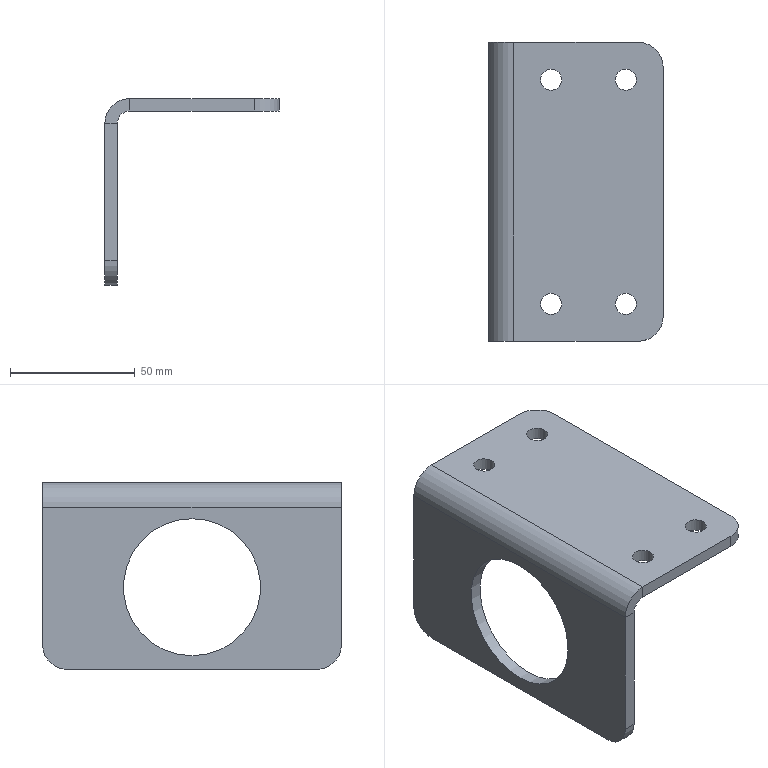Part | STEP file | JBJ-P-1007-02 | 1 solid | 23 faces | box 70 x 120 x 75 mm | volume 68625 mm3 | plane 12 | cylinder 11 | commonest cylinder face diameters 20 x5 8.5 x4 10 x1 55 x1
STEP:
#1=CARTESIAN_POINT('',(10.,-120.,75.));
#2=VERTEX_POINT('',#1);
#3=CARTESIAN_POINT('',(10.,-120.,70.));
#4=VERTEX_POINT('',#3);
#5=CARTESIAN_POINT('',(10.,-120.,75.));
#6=DIRECTION('',(0.,0.,-1.));
#7=VECTOR('',#6,1000.);
#8=LINE('',#5,#7);
#9=EDGE_CURVE('',#2,#4,#8,.T.);
#10=ORIENTED_EDGE('',*,*,#9,.F.);
#11=CARTESIAN_POINT('',(0.,-120.,65.));
#12=VERTEX_POINT('',#11);
#13=CARTESIAN_POINT('',(10.,-120.,65.));
#14=DIRECTION('',(0.,1.,0.));
#15=DIRECTION('',(0.,0.,-1.));
#16=AXIS2_PLACEMENT_3D('',#13,#14,#15);
#17=CIRCLE('',#16,10.);
#18=EDGE_CURVE('',#12,#2,#17,.T.);
#19=ORIENTED_EDGE('',*,*,#18,.F.);
#20=CARTESIAN_POINT('',(5.,-120.,65.));
#21=VERTEX_POINT('',#20);
#22=CARTESIAN_POINT('',(5.,-120.,65.));
#23=DIRECTION('',(-1.,0.,0.));
#24=VECTOR('',#23,1000.);
#25=LINE('',#22,#24);
#26=EDGE_CURVE('',#21,#12,#25,.T.);
#27=ORIENTED_EDGE('',*,*,#26,.F.);
#28=CARTESIAN_POINT('',(10.,-120.,65.));
#29=DIRECTION('',(0.,1.,0.));
#30=DIRECTION('',(1.,0.,0.));
#31=AXIS2_PLACEMENT_3D('',#28,#29,#30);
#32=CIRCLE('',#31,5.);
#33=EDGE_CURVE('',#21,#4,#32,.T.);
#34=ORIENTED_EDGE('',*,*,#33,.T.);
#35=EDGE_LOOP('',(#10,#19,#27,#34));
#36=FACE_OUTER_BOUND('',#35,.T.);
#37=CARTESIAN_POINT('',(10.,-120.,75.));
#38=DIRECTION('',(0.,-1.,0.));
#39=DIRECTION('',(0.,0.,-1.));
#40=AXIS2_PLACEMENT_3D('',#37,#38,#39);
#41=PLANE('',#40);
#42=ADVANCED_FACE('',(#36),#41,.T.);
#43=CARTESIAN_POINT('',(60.,-120.,70.));
#44=VERTEX_POINT('',#43);
#45=CARTESIAN_POINT('',(0.,-120.,70.));
#46=DIRECTION('',(1.,0.,0.));
#47=VECTOR('',#46,1000.);
#48=LINE('',#45,#47);
#49=EDGE_CURVE('',#4,#44,#48,.T.);
#50=ORIENTED_EDGE('',*,*,#49,.T.);
#51=CARTESIAN_POINT('',(60.,-120.,75.));
#52=VERTEX_POINT('',#51);
#53=CARTESIAN_POINT('',(60.,-120.,75.));
#54=DIRECTION('',(0.,0.,1.));
#55=VECTOR('',#54,1000.);
#56=LINE('',#53,#55);
#57=EDGE_CURVE('',#44,#52,#56,.T.);
#58=ORIENTED_EDGE('',*,*,#57,.T.);
#59=CARTESIAN_POINT('',(0.,-120.,75.));
#60=DIRECTION('',(1.,0.,0.));
#61=VECTOR('',#60,1000.);
#62=LINE('',#59,#61);
#63=EDGE_CURVE('',#2,#52,#62,.T.);
#64=ORIENTED_EDGE('',*,*,#63,.F.);
#65=ORIENTED_EDGE('',*,*,#9,.T.);
#66=EDGE_LOOP('',(#50,#58,#64,#65));
#67=FACE_OUTER_BOUND('',#66,.T.);
#68=CARTESIAN_POINT('',(5.,-120.,65.));
#69=DIRECTION('',(0.,-1.,0.));
#70=DIRECTION('',(0.,0.,-1.));
#71=AXIS2_PLACEMENT_3D('',#68,#69,#70);
#72=PLANE('',#71);
#73=ADVANCED_FACE('',(#67),#72,.T.);
#74=CARTESIAN_POINT('',(0.,0.,65.));
#75=VERTEX_POINT('',#74);
#76=CARTESIAN_POINT('',(5.,0.,65.));
#77=VERTEX_POINT('',#76);
#78=CARTESIAN_POINT('',(0.,0.,65.));
#79=DIRECTION('',(1.,0.,0.));
#80=VECTOR('',#79,1000.);
#81=LINE('',#78,#80);
#82=EDGE_CURVE('',#75,#77,#81,.T.);
#83=ORIENTED_EDGE('',*,*,#82,.F.);
#84=CARTESIAN_POINT('',(10.,0.,75.));
#85=VERTEX_POINT('',#84);
#86=CARTESIAN_POINT('',(10.,0.,65.));
#87=DIRECTION('',(0.,1.,0.));
#88=DIRECTION('',(0.,0.,-1.));
#89=AXIS2_PLACEMENT_3D('',#86,#87,#88);
#90=CIRCLE('',#89,10.);
#91=EDGE_CURVE('',#75,#85,#90,.T.);
#92=ORIENTED_EDGE('',*,*,#91,.T.);
#93=CARTESIAN_POINT('',(10.,0.,70.));
#94=VERTEX_POINT('',#93);
#95=CARTESIAN_POINT('',(10.,0.,70.));
#96=DIRECTION('',(0.,0.,1.));
#97=VECTOR('',#96,1000.);
#98=LINE('',#95,#97);
#99=EDGE_CURVE('',#94,#85,#98,.T.);
#100=ORIENTED_EDGE('',*,*,#99,.F.);
#101=CARTESIAN_POINT('',(10.,0.,65.));
#102=DIRECTION('',(0.,1.,0.));
#103=DIRECTION('',(1.,0.,0.));
#104=AXIS2_PLACEMENT_3D('',#101,#102,#103);
#105=CIRCLE('',#104,5.);
#106=EDGE_CURVE('',#77,#94,#105,.T.);
#107=ORIENTED_EDGE('',*,*,#106,.F.);
#108=EDGE_LOOP('',(#83,#92,#100,#107));
#109=FACE_OUTER_BOUND('',#108,.T.);
#110=CARTESIAN_POINT('',(0.,0.,65.));
#111=DIRECTION('',(0.,1.,0.));
#112=DIRECTION('',(0.,0.,1.));
#113=AXIS2_PLACEMENT_3D('',#110,#111,#112);
#114=PLANE('',#113);
#115=ADVANCED_FACE('',(#109),#114,.T.);
#116=CARTESIAN_POINT('',(5.,0.,10.));
#117=VERTEX_POINT('',#116);
#118=CARTESIAN_POINT('',(5.,0.,0.));
#119=DIRECTION('',(0.,0.,1.));
#120=VECTOR('',#119,1000.);
#121=LINE('',#118,#120);
#122=EDGE_CURVE('',#117,#77,#121,.T.);
#123=ORIENTED_EDGE('',*,*,#122,.F.);
#124=CARTESIAN_POINT('',(0.,0.,10.));
#125=VERTEX_POINT('',#124);
#126=CARTESIAN_POINT('',(0.,0.,10.));
#127=DIRECTION('',(-1.,0.,0.));
#128=VECTOR('',#127,1000.);
#129=LINE('',#126,#128);
#130=EDGE_CURVE('',#117,#125,#129,.T.);
#131=ORIENTED_EDGE('',*,*,#130,.T.);
#132=CARTESIAN_POINT('',(0.,0.,0.));
#133=DIRECTION('',(0.,0.,1.));
#134=VECTOR('',#133,1000.);
#135=LINE('',#132,#134);
#136=EDGE_CURVE('',#125,#75,#135,.T.);
#137=ORIENTED_EDGE('',*,*,#136,.T.);
#138=ORIENTED_EDGE('',*,*,#82,.T.);
#139=EDGE_LOOP('',(#123,#131,#137,#138));
#140=FACE_OUTER_BOUND('',#139,.T.);
#141=CARTESIAN_POINT('',(10.,0.,70.));
#142=DIRECTION('',(0.,1.,0.));
#143=DIRECTION('',(0.,0.,1.));
#144=AXIS2_PLACEMENT_3D('',#141,#142,#143);
#145=PLANE('',#144);
#146=ADVANCED_FACE('',(#140),#145,.T.);
#147=CARTESIAN_POINT('',(50.75,-15.,75.));
#148=VERTEX_POINT('',#147);
#149=CARTESIAN_POINT('',(55.,-15.,75.));
#150=DIRECTION('',(0.,0.,-1.));
#151=DIRECTION('',(-1.,0.,0.));
#152=AXIS2_PLACEMENT_3D('',#149,#150,#151);
#153=CIRCLE('',#152,4.25);
#154=EDGE_CURVE('',#148,#148,#153,.T.);
#155=ORIENTED_EDGE('',*,*,#154,.T.);
#156=EDGE_LOOP('',(#155));
#157=FACE_BOUND('',#156,.T.);
#158=CARTESIAN_POINT('',(20.75,-15.,75.));
#159=VERTEX_POINT('',#158);
#160=CARTESIAN_POINT('',(25.,-15.,75.));
#161=DIRECTION('',(0.,0.,-1.));
#162=DIRECTION('',(-1.,0.,0.));
#163=AXIS2_PLACEMENT_3D('',#160,#161,#162);
#164=CIRCLE('',#163,4.25);
#165=EDGE_CURVE('',#159,#159,#164,.T.);
#166=ORIENTED_EDGE('',*,*,#165,.T.);
#167=EDGE_LOOP('',(#166));
#168=FACE_BOUND('',#167,.T.);
#169=CARTESIAN_POINT('',(50.75,-105.,75.));
#170=VERTEX_POINT('',#169);
#171=CARTESIAN_POINT('',(55.,-105.,75.));
#172=DIRECTION('',(0.,0.,-1.));
#173=DIRECTION('',(-1.,0.,0.));
#174=AXIS2_PLACEMENT_3D('',#171,#172,#173);
#175=CIRCLE('',#174,4.25);
#176=EDGE_CURVE('',#170,#170,#175,.T.);
#177=ORIENTED_EDGE('',*,*,#176,.T.);
#178=EDGE_LOOP('',(#177));
#179=FACE_BOUND('',#178,.T.);
#180=CARTESIAN_POINT('',(20.75,-105.,75.));
#181=VERTEX_POINT('',#180);
#182=CARTESIAN_POINT('',(25.,-105.,75.));
#183=DIRECTION('',(0.,0.,-1.));
#184=DIRECTION('',(-1.,0.,0.));
#185=AXIS2_PLACEMENT_3D('',#182,#183,#184);
#186=CIRCLE('',#185,4.25);
#187=EDGE_CURVE('',#181,#181,#186,.T.);
#188=ORIENTED_EDGE('',*,*,#187,.T.);
#189=EDGE_LOOP('',(#188));
#190=FACE_BOUND('',#189,.T.);
#191=CARTESIAN_POINT('',(70.,-110.,75.));
#192=VERTEX_POINT('',#191);
#193=CARTESIAN_POINT('',(70.,-10.,75.));
#194=VERTEX_POINT('',#193);
#195=CARTESIAN_POINT('',(70.,-120.,75.));
#196=DIRECTION('',(0.,1.,0.));
#197=VECTOR('',#196,1000.);
#198=LINE('',#195,#197);
#199=EDGE_CURVE('',#192,#194,#198,.T.);
#200=ORIENTED_EDGE('',*,*,#199,.T.);
#201=CARTESIAN_POINT('',(60.,0.,75.));
#202=VERTEX_POINT('',#201);
#203=CARTESIAN_POINT('',(60.,-10.,75.));
#204=DIRECTION('',(0.,0.,1.));
#205=DIRECTION('',(1.,0.,0.));
#206=AXIS2_PLACEMENT_3D('',#203,#204,#205);
#207=CIRCLE('',#206,10.);
#208=EDGE_CURVE('',#194,#202,#207,.T.);
#209=ORIENTED_EDGE('',*,*,#208,.T.);
#210=CARTESIAN_POINT('',(0.,0.,75.));
#211=DIRECTION('',(1.,0.,0.));
#212=VECTOR('',#211,1000.);
#213=LINE('',#210,#212);
#214=EDGE_CURVE('',#85,#202,#213,.T.);
#215=ORIENTED_EDGE('',*,*,#214,.F.);
#216=CARTESIAN_POINT('',(10.,-120.,75.));
#217=DIRECTION('',(0.,1.,0.));
#218=VECTOR('',#217,1000.);
#219=LINE('',#216,#218);
#220=EDGE_CURVE('',#2,#85,#219,.T.);
#221=ORIENTED_EDGE('',*,*,#220,.F.);
#222=ORIENTED_EDGE('',*,*,#63,.T.);
#223=CARTESIAN_POINT('',(60.,-110.,75.));
#224=DIRECTION('',(0.,0.,1.));
#225=DIRECTION('',(1.,0.,0.));
#226=AXIS2_PLACEMENT_3D('',#223,#224,#225);
#227=CIRCLE('',#226,10.);
#228=EDGE_CURVE('',#52,#192,#227,.T.);
#229=ORIENTED_EDGE('',*,*,#228,.T.);
#230=EDGE_LOOP('',(#200,#209,#215,#221,#222,#229));
#231=FACE_OUTER_BOUND('',#230,.T.);
#232=CARTESIAN_POINT('',(0.,-120.,75.));
#233=DIRECTION('',(0.,0.,1.));
#234=DIRECTION('',(1.,0.,0.));
#235=AXIS2_PLACEMENT_3D('',#232,#233,#234);
#236=PLANE('',#235);
#237=ADVANCED_FACE('',(#157,#168,#179,#190,#231),#236,.T.);
#238=ORIENTED_EDGE('',*,*,#91,.F.);
#239=CARTESIAN_POINT('',(0.,-120.,65.));
#240=DIRECTION('',(0.,1.,0.));
#241=VECTOR('',#240,1000.);
#242=LINE('',#239,#241);
#243=EDGE_CURVE('',#12,#75,#242,.T.);
#244=ORIENTED_EDGE('',*,*,#243,.F.);
#245=ORIENTED_EDGE('',*,*,#18,.T.);
#246=ORIENTED_EDGE('',*,*,#220,.T.);
#247=EDGE_LOOP('',(#238,#244,#245,#246));
#248=FACE_OUTER_BOUND('',#247,.T.);
#249=CARTESIAN_POINT('',(10.,-120.,65.));
#250=DIRECTION('',(0.,1.,0.));
#251=DIRECTION('',(0.,0.,1.));
#252=AXIS2_PLACEMENT_3D('',#249,#250,#251);
#253=CYLINDRICAL_SURFACE('',#252,10.);
#254=ADVANCED_FACE('',(#248),#253,.T.);
#255=CARTESIAN_POINT('',(0.,-60.,5.5));
#256=VERTEX_POINT('',#255);
#257=CARTESIAN_POINT('',(0.,-60.,33.));
#258=DIRECTION('',(1.,0.,0.));
#259=DIRECTION('',(0.,0.,-1.));
#260=AXIS2_PLACEMENT_3D('',#257,#258,#259);
#261=CIRCLE('',#260,27.5);
#262=EDGE_CURVE('',#256,#256,#261,.T.);
#263=ORIENTED_EDGE('',*,*,#262,.T.);
#264=EDGE_LOOP('',(#263));
#265=FACE_BOUND('',#264,.T.);
#266=CARTESIAN_POINT('',(0.,-110.,0.));
#267=VERTEX_POINT('',#266);
#268=CARTESIAN_POINT('',(0.,-10.,0.));
#269=VERTEX_POINT('',#268);
#270=CARTESIAN_POINT('',(0.,-120.,0.));
#271=DIRECTION('',(0.,1.,0.));
#272=VECTOR('',#271,1000.);
#273=LINE('',#270,#272);
#274=EDGE_CURVE('',#267,#269,#273,.T.);
#275=ORIENTED_EDGE('',*,*,#274,.F.);
#276=CARTESIAN_POINT('',(0.,-120.,10.));
#277=VERTEX_POINT('',#276);
#278=CARTESIAN_POINT('',(0.,-110.,10.));
#279=DIRECTION('',(-1.,0.,0.));
#280=DIRECTION('',(0.,0.,1.));
#281=AXIS2_PLACEMENT_3D('',#278,#279,#280);
#282=CIRCLE('',#281,10.);
#283=EDGE_CURVE('',#267,#277,#282,.T.);
#284=ORIENTED_EDGE('',*,*,#283,.T.);
#285=CARTESIAN_POINT('',(0.,-120.,0.));
#286=DIRECTION('',(0.,0.,1.));
#287=VECTOR('',#286,1000.);
#288=LINE('',#285,#287);
#289=EDGE_CURVE('',#277,#12,#288,.T.);
#290=ORIENTED_EDGE('',*,*,#289,.T.);
#291=ORIENTED_EDGE('',*,*,#243,.T.);
#292=ORIENTED_EDGE('',*,*,#136,.F.);
#293=CARTESIAN_POINT('',(0.,-10.,10.));
#294=DIRECTION('',(-1.,0.,0.));
#295=DIRECTION('',(0.,0.,1.));
#296=AXIS2_PLACEMENT_3D('',#293,#294,#295);
#297=CIRCLE('',#296,10.);
#298=EDGE_CURVE('',#125,#269,#297,.T.);
#299=ORIENTED_EDGE('',*,*,#298,.T.);
#300=EDGE_LOOP('',(#275,#284,#290,#291,#292,#299));
#301=FACE_OUTER_BOUND('',#300,.T.);
#302=CARTESIAN_POINT('',(0.,-120.,0.));
#303=DIRECTION('',(-1.,0.,0.));
#304=DIRECTION('',(0.,0.,1.));
#305=AXIS2_PLACEMENT_3D('',#302,#303,#304);
#306=PLANE('',#305);
#307=ADVANCED_FACE('',(#265,#301),#306,.T.);
#308=CARTESIAN_POINT('',(5.,-110.,0.));
#309=VERTEX_POINT('',#308);
#310=CARTESIAN_POINT('',(5.,-10.,0.));
#311=VERTEX_POINT('',#310);
#312=CARTESIAN_POINT('',(5.,-120.,0.));
#313=DIRECTION('',(0.,1.,0.));
#314=VECTOR('',#313,1000.);
#315=LINE('',#312,#314);
#316=EDGE_CURVE('',#309,#311,#315,.T.);
#317=ORIENTED_EDGE('',*,*,#316,.F.);
#318=CARTESIAN_POINT('',(0.,-110.,0.));
#319=DIRECTION('',(-1.,0.,0.));
#320=VECTOR('',#319,1000.);
#321=LINE('',#318,#320);
#322=EDGE_CURVE('',#309,#267,#321,.T.);
#323=ORIENTED_EDGE('',*,*,#322,.T.);
#324=ORIENTED_EDGE('',*,*,#274,.T.);
#325=CARTESIAN_POINT('',(5.,-10.,0.));
#326=DIRECTION('',(1.,0.,0.));
#327=VECTOR('',#326,1000.);
#328=LINE('',#325,#327);
#329=EDGE_CURVE('',#269,#311,#328,.T.);
#330=ORIENTED_EDGE('',*,*,#329,.T.);
#331=EDGE_LOOP('',(#317,#323,#324,#330));
#332=FACE_OUTER_BOUND('',#331,.T.);
#333=CARTESIAN_POINT('',(0.,-120.,0.));
#334=DIRECTION('',(0.,0.,1.));
#335=DIRECTION('',(1.,0.,0.));
#336=AXIS2_PLACEMENT_3D('',#333,#334,#335);
#337=PLANE('',#336);
#338=ADVANCED_FACE('',(#332),#337,.F.);
#339=CARTESIAN_POINT('',(5.,-60.,5.5));
#340=VERTEX_POINT('',#339);
#341=CARTESIAN_POINT('',(5.,-60.,33.));
#342=DIRECTION('',(1.,0.,0.));
#343=DIRECTION('',(0.,0.,-1.));
#344=AXIS2_PLACEMENT_3D('',#341,#342,#343);
#345=CIRCLE('',#344,27.5);
#346=EDGE_CURVE('',#340,#340,#345,.T.);
#347=ORIENTED_EDGE('',*,*,#346,.F.);
#348=EDGE_LOOP('',(#347));
#349=FACE_BOUND('',#348,.T.);
#350=CARTESIAN_POINT('',(5.,-120.,10.));
#351=VERTEX_POINT('',#350);
#352=CARTESIAN_POINT('',(5.,-120.,0.));
#353=DIRECTION('',(0.,0.,1.));
#354=VECTOR('',#353,1000.);
#355=LINE('',#352,#354);
#356=EDGE_CURVE('',#351,#21,#355,.T.);
#357=ORIENTED_EDGE('',*,*,#356,.F.);
#358=CARTESIAN_POINT('',(5.,-110.,10.));
#359=DIRECTION('',(1.,0.,0.));
#360=DIRECTION('',(0.,0.,1.));
#361=AXIS2_PLACEMENT_3D('',#358,#359,#360);
#362=CIRCLE('',#361,10.);
#363=EDGE_CURVE('',#351,#309,#362,.T.);
#364=ORIENTED_EDGE('',*,*,#363,.T.);
#365=ORIENTED_EDGE('',*,*,#316,.T.);
#366=CARTESIAN_POINT('',(5.,-10.,10.));
#367=DIRECTION('',(1.,0.,0.));
#368=DIRECTION('',(0.,0.,1.));
#369=AXIS2_PLACEMENT_3D('',#366,#367,#368);
#370=CIRCLE('',#369,10.);
#371=EDGE_CURVE('',#311,#117,#370,.T.);
#372=ORIENTED_EDGE('',*,*,#371,.T.);
#373=ORIENTED_EDGE('',*,*,#122,.T.);
#374=CARTESIAN_POINT('',(5.,-120.,65.));
#375=DIRECTION('',(0.,1.,0.));
#376=VECTOR('',#375,1000.);
#377=LINE('',#374,#376);
#378=EDGE_CURVE('',#21,#77,#377,.T.);
#379=ORIENTED_EDGE('',*,*,#378,.F.);
#380=EDGE_LOOP('',(#357,#364,#365,#372,#373,#379));
#381=FACE_OUTER_BOUND('',#380,.T.);
#382=CARTESIAN_POINT('',(5.,-120.,0.));
#383=DIRECTION('',(-1.,0.,0.));
#384=DIRECTION('',(0.,0.,1.));
#385=AXIS2_PLACEMENT_3D('',#382,#383,#384);
#386=PLANE('',#385);
#387=ADVANCED_FACE('',(#349,#381),#386,.F.);
#388=ORIENTED_EDGE('',*,*,#106,.T.);
#389=CARTESIAN_POINT('',(10.,-120.,70.));
#390=DIRECTION('',(0.,1.,0.));
#391=VECTOR('',#390,1000.);
#392=LINE('',#389,#391);
#393=EDGE_CURVE('',#4,#94,#392,.T.);
#394=ORIENTED_EDGE('',*,*,#393,.F.);
#395=ORIENTED_EDGE('',*,*,#33,.F.);
#396=ORIENTED_EDGE('',*,*,#378,.T.);
#397=EDGE_LOOP('',(#388,#394,#395,#396));
#398=FACE_OUTER_BOUND('',#397,.T.);
#399=CARTESIAN_POINT('',(10.,-120.,65.));
#400=DIRECTION('',(0.,1.,0.));
#401=DIRECTION('',(0.,0.,1.));
#402=AXIS2_PLACEMENT_3D('',#399,#400,#401);
#403=CYLINDRICAL_SURFACE('',#402,5.);
#404=ADVANCED_FACE('',(#398),#403,.F.);
#405=CARTESIAN_POINT('',(50.75,-15.,70.));
#406=VERTEX_POINT('',#405);
#407=CARTESIAN_POINT('',(55.,-15.,70.));
#408=DIRECTION('',(0.,0.,-1.));
#409=DIRECTION('',(-1.,0.,0.));
#410=AXIS2_PLACEMENT_3D('',#407,#408,#409);
#411=CIRCLE('',#410,4.25);
#412=EDGE_CURVE('',#406,#406,#411,.T.);
#413=ORIENTED_EDGE('',*,*,#412,.F.);
#414=EDGE_LOOP('',(#413));
#415=FACE_BOUND('',#414,.T.);
#416=CARTESIAN_POINT('',(20.75,-15.,70.));
#417=VERTEX_POINT('',#416);
#418=CARTESIAN_POINT('',(25.,-15.,70.));
#419=DIRECTION('',(0.,0.,-1.));
#420=DIRECTION('',(-1.,0.,0.));
#421=AXIS2_PLACEMENT_3D('',#418,#419,#420);
#422=CIRCLE('',#421,4.25);
#423=EDGE_CURVE('',#417,#417,#422,.T.);
#424=ORIENTED_EDGE('',*,*,#423,.F.);
#425=EDGE_LOOP('',(#424));
#426=FACE_BOUND('',#425,.T.);
#427=CARTESIAN_POINT('',(50.75,-105.,70.));
#428=VERTEX_POINT('',#427);
#429=CARTESIAN_POINT('',(55.,-105.,70.));
#430=DIRECTION('',(0.,0.,-1.));
#431=DIRECTION('',(-1.,0.,0.));
#432=AXIS2_PLACEMENT_3D('',#429,#430,#431);
#433=CIRCLE('',#432,4.25);
#434=EDGE_CURVE('',#428,#428,#433,.T.);
#435=ORIENTED_EDGE('',*,*,#434,.F.);
#436=EDGE_LOOP('',(#435));
#437=FACE_BOUND('',#436,.T.);
#438=CARTESIAN_POINT('',(20.75,-105.,70.));
#439=VERTEX_POINT('',#438);
#440=CARTESIAN_POINT('',(25.,-105.,70.));
#441=DIRECTION('',(0.,0.,-1.));
#442=DIRECTION('',(-1.,0.,0.));
#443=AXIS2_PLACEMENT_3D('',#440,#441,#442);
#444=CIRCLE('',#443,4.25);
#445=EDGE_CURVE('',#439,#439,#444,.T.);
#446=ORIENTED_EDGE('',*,*,#445,.F.);
#447=EDGE_LOOP('',(#446));
#448=FACE_BOUND('',#447,.T.);
#449=CARTESIAN_POINT('',(60.,0.,70.));
#450=VERTEX_POINT('',#449);
#451=CARTESIAN_POINT('',(0.,0.,70.));
#452=DIRECTION('',(1.,0.,0.));
#453=VECTOR('',#452,1000.);
#454=LINE('',#451,#453);
#455=EDGE_CURVE('',#94,#450,#454,.T.);
#456=ORIENTED_EDGE('',*,*,#455,.T.);
#457=CARTESIAN_POINT('',(70.,-10.,70.));
#458=VERTEX_POINT('',#457);
#459=CARTESIAN_POINT('',(60.,-10.,70.));
#460=DIRECTION('',(0.,0.,-1.));
#461=DIRECTION('',(1.,0.,0.));
#462=AXIS2_PLACEMENT_3D('',#459,#460,#461);
#463=CIRCLE('',#462,10.);
#464=EDGE_CURVE('',#450,#458,#463,.T.);
#465=ORIENTED_EDGE('',*,*,#464,.T.);
#466=CARTESIAN_POINT('',(70.,-110.,70.));
#467=VERTEX_POINT('',#466);
#468=CARTESIAN_POINT('',(70.,-120.,70.));
#469=DIRECTION('',(0.,1.,0.));
#470=VECTOR('',#469,1000.);
#471=LINE('',#468,#470);
#472=EDGE_CURVE('',#467,#458,#471,.T.);
#473=ORIENTED_EDGE('',*,*,#472,.F.);
#474=CARTESIAN_POINT('',(60.,-110.,70.));
#475=DIRECTION('',(0.,0.,-1.));
#476=DIRECTION('',(1.,0.,0.));
#477=AXIS2_PLACEMENT_3D('',#474,#475,#476);
#478=CIRCLE('',#477,10.);
#479=EDGE_CURVE('',#467,#44,#478,.T.);
#480=ORIENTED_EDGE('',*,*,#479,.T.);
#481=ORIENTED_EDGE('',*,*,#49,.F.);
#482=ORIENTED_EDGE('',*,*,#393,.T.);
#483=EDGE_LOOP('',(#456,#465,#473,#480,#481,#482));
#484=FACE_OUTER_BOUND('',#483,.T.);
#485=CARTESIAN_POINT('',(0.,-120.,70.));
#486=DIRECTION('',(0.,0.,1.));
#487=DIRECTION('',(1.,0.,0.));
#488=AXIS2_PLACEMENT_3D('',#485,#486,#487);
#489=PLANE('',#488);
#490=ADVANCED_FACE('',(#415,#426,#437,#448,#484),#489,.F.);
#491=ORIENTED_EDGE('',*,*,#472,.T.);
#492=CARTESIAN_POINT('',(70.,-10.,75.));
#493=DIRECTION('',(0.,0.,1.));
#494=VECTOR('',#493,1000.);
#495=LINE('',#492,#494);
#496=EDGE_CURVE('',#458,#194,#495,.T.);
#497=ORIENTED_EDGE('',*,*,#496,.T.);
#498=ORIENTED_EDGE('',*,*,#199,.F.);
#499=CARTESIAN_POINT('',(70.,-110.,70.));
#500=DIRECTION('',(0.,0.,-1.));
#501=VECTOR('',#500,1000.);
#502=LINE('',#499,#501);
#503=EDGE_CURVE('',#192,#467,#502,.T.);
#504=ORIENTED_EDGE('',*,*,#503,.T.);
#505=EDGE_LOOP('',(#491,#497,#498,#504));
#506=FACE_OUTER_BOUND('',#505,.T.);
#507=CARTESIAN_POINT('',(70.,-120.,70.));
#508=DIRECTION('',(-1.,0.,0.));
#509=DIRECTION('',(0.,0.,1.));
#510=AXIS2_PLACEMENT_3D('',#507,#508,#509);
#511=PLANE('',#510);
#512=ADVANCED_FACE('',(#506),#511,.F.);
#513=ORIENTED_EDGE('',*,*,#289,.F.);
#514=CARTESIAN_POINT('',(10.,-120.,10.));
#515=DIRECTION('',(1.,0.,0.));
#516=VECTOR('',#515,1000.);
#517=LINE('',#514,#516);
#518=EDGE_CURVE('',#277,#351,#517,.T.);
#519=ORIENTED_EDGE('',*,*,#518,.T.);
#520=ORIENTED_EDGE('',*,*,#356,.T.);
#521=ORIENTED_EDGE('',*,*,#26,.T.);
#522=EDGE_LOOP('',(#513,#519,#520,#521));
#523=FACE_OUTER_BOUND('',#522,.T.);
#524=CARTESIAN_POINT('',(10.,-120.,65.));
#525=DIRECTION('',(0.,1.,0.));
#526=DIRECTION('',(1.,0.,0.));
#527=AXIS2_PLACEMENT_3D('',#524,#525,#526);
#528=PLANE('',#527);
#529=ADVANCED_FACE('',(#523),#528,.F.);
#530=ORIENTED_EDGE('',*,*,#214,.T.);
#531=CARTESIAN_POINT('',(60.,0.,70.));
#532=DIRECTION('',(0.,0.,-1.));
#533=VECTOR('',#532,1000.);
#534=LINE('',#531,#533);
#535=EDGE_CURVE('',#202,#450,#534,.T.);
#536=ORIENTED_EDGE('',*,*,#535,.T.);
#537=ORIENTED_EDGE('',*,*,#455,.F.);
#538=ORIENTED_EDGE('',*,*,#99,.T.);
#539=EDGE_LOOP('',(#530,#536,#537,#538));
#540=FACE_OUTER_BOUND('',#539,.T.);
#541=CARTESIAN_POINT('',(10.,0.,65.));
#542=DIRECTION('',(0.,1.,0.));
#543=DIRECTION('',(1.,0.,0.));
#544=AXIS2_PLACEMENT_3D('',#541,#542,#543);
#545=PLANE('',#544);
#546=ADVANCED_FACE('',(#540),#545,.T.);
#547=ORIENTED_EDGE('',*,*,#464,.F.);
#548=ORIENTED_EDGE('',*,*,#535,.F.);
#549=ORIENTED_EDGE('',*,*,#208,.F.);
#550=ORIENTED_EDGE('',*,*,#496,.F.);
#551=EDGE_LOOP('',(#547,#548,#549,#550));
#552=FACE_OUTER_BOUND('',#551,.T.);
#553=CARTESIAN_POINT('',(60.,-10.,70.));
#554=DIRECTION('',(0.,0.,-1.));
#555=DIRECTION('',(-1.,0.,0.));
#556=AXIS2_PLACEMENT_3D('',#553,#554,#555);
#557=CYLINDRICAL_SURFACE('',#556,10.);
#558=ADVANCED_FACE('',(#552),#557,.T.);
#559=ORIENTED_EDGE('',*,*,#479,.F.);
#560=ORIENTED_EDGE('',*,*,#503,.F.);
#561=ORIENTED_EDGE('',*,*,#228,.F.);
#562=ORIENTED_EDGE('',*,*,#57,.F.);
#563=EDGE_LOOP('',(#559,#560,#561,#562));
#564=FACE_OUTER_BOUND('',#563,.T.);
#565=CARTESIAN_POINT('',(60.,-110.,65.));
#566=DIRECTION('',(0.,0.,-1.));
#567=DIRECTION('',(-1.,0.,0.));
#568=AXIS2_PLACEMENT_3D('',#565,#566,#567);
#569=CYLINDRICAL_SURFACE('',#568,10.);
#570=ADVANCED_FACE('',(#564),#569,.T.);
#571=ORIENTED_EDGE('',*,*,#283,.F.);
#572=ORIENTED_EDGE('',*,*,#322,.F.);
#573=ORIENTED_EDGE('',*,*,#363,.F.);
#574=ORIENTED_EDGE('',*,*,#518,.F.);
#575=EDGE_LOOP('',(#571,#572,#573,#574));
#576=FACE_OUTER_BOUND('',#575,.T.);
#577=CARTESIAN_POINT('',(10.,-110.,10.));
#578=DIRECTION('',(1.,0.,0.));
#579=DIRECTION('',(0.,0.,-1.));
#580=AXIS2_PLACEMENT_3D('',#577,#578,#579);
#581=CYLINDRICAL_SURFACE('',#580,10.);
#582=ADVANCED_FACE('',(#576),#581,.T.);
#583=ORIENTED_EDGE('',*,*,#298,.F.);
#584=ORIENTED_EDGE('',*,*,#130,.F.);
#585=ORIENTED_EDGE('',*,*,#371,.F.);
#586=ORIENTED_EDGE('',*,*,#329,.F.);
#587=EDGE_LOOP('',(#583,#584,#585,#586));
#588=FACE_OUTER_BOUND('',#587,.T.);
#589=CARTESIAN_POINT('',(0.,-10.,10.));
#590=DIRECTION('',(-1.,0.,0.));
#591=DIRECTION('',(0.,0.,1.));
#592=AXIS2_PLACEMENT_3D('',#589,#590,#591);
#593=CYLINDRICAL_SURFACE('',#592,10.);
#594=ADVANCED_FACE('',(#588),#593,.T.);
#595=ORIENTED_EDGE('',*,*,#262,.F.);
#596=EDGE_LOOP('',(#595));
#597=FACE_OUTER_BOUND('',#596,.T.);
#598=ORIENTED_EDGE('',*,*,#346,.T.);
#599=EDGE_LOOP('',(#598));
#600=FACE_OUTER_BOUND('',#599,.T.);
#601=CARTESIAN_POINT('',(0.,-60.,33.));
#602=DIRECTION('',(1.,0.,0.));
#603=DIRECTION('',(0.,0.,-1.));
#604=AXIS2_PLACEMENT_3D('',#601,#602,#603);
#605=CYLINDRICAL_SURFACE('',#604,27.5);
#606=ADVANCED_FACE('',(#597,#600),#605,.F.);
#607=ORIENTED_EDGE('',*,*,#187,.F.);
#608=EDGE_LOOP('',(#607));
#609=FACE_OUTER_BOUND('',#608,.T.);
#610=ORIENTED_EDGE('',*,*,#445,.T.);
#611=EDGE_LOOP('',(#610));
#612=FACE_OUTER_BOUND('',#611,.T.);
#613=CARTESIAN_POINT('',(25.,-105.,70.));
#614=DIRECTION('',(0.,0.,-1.));
#615=DIRECTION('',(-1.,0.,0.));
#616=AXIS2_PLACEMENT_3D('',#613,#614,#615);
#617=CYLINDRICAL_SURFACE('',#616,4.25);
#618=ADVANCED_FACE('',(#609,#612),#617,.F.);
#619=ORIENTED_EDGE('',*,*,#176,.F.);
#620=EDGE_LOOP('',(#619));
#621=FACE_OUTER_BOUND('',#620,.T.);
#622=ORIENTED_EDGE('',*,*,#434,.T.);
#623=EDGE_LOOP('',(#622));
#624=FACE_OUTER_BOUND('',#623,.T.);
#625=CARTESIAN_POINT('',(55.,-105.,70.));
#626=DIRECTION('',(0.,0.,-1.));
#627=DIRECTION('',(-1.,0.,0.));
#628=AXIS2_PLACEMENT_3D('',#625,#626,#627);
#629=CYLINDRICAL_SURFACE('',#628,4.25);
#630=ADVANCED_FACE('',(#621,#624),#629,.F.);
#631=ORIENTED_EDGE('',*,*,#165,.F.);
#632=EDGE_LOOP('',(#631));
#633=FACE_OUTER_BOUND('',#632,.T.);
#634=ORIENTED_EDGE('',*,*,#423,.T.);
#635=EDGE_LOOP('',(#634));
#636=FACE_OUTER_BOUND('',#635,.T.);
#637=CARTESIAN_POINT('',(25.,-15.,70.));
#638=DIRECTION('',(0.,0.,-1.));
#639=DIRECTION('',(-1.,0.,0.));
#640=AXIS2_PLACEMENT_3D('',#637,#638,#639);
#641=CYLINDRICAL_SURFACE('',#640,4.25);
#642=ADVANCED_FACE('',(#633,#636),#641,.F.);
#643=ORIENTED_EDGE('',*,*,#154,.F.);
#644=EDGE_LOOP('',(#643));
#645=FACE_OUTER_BOUND('',#644,.T.);
#646=ORIENTED_EDGE('',*,*,#412,.T.);
#647=EDGE_LOOP('',(#646));
#648=FACE_OUTER_BOUND('',#647,.T.);
#649=CARTESIAN_POINT('',(55.,-15.,70.));
#650=DIRECTION('',(0.,0.,-1.));
#651=DIRECTION('',(-1.,0.,0.));
#652=AXIS2_PLACEMENT_3D('',#649,#650,#651);
#653=CYLINDRICAL_SURFACE('',#652,4.25);
#654=ADVANCED_FACE('',(#645,#648),#653,.F.);
#655=CLOSED_SHELL('',(#42,#73,#115,#146,#237,#254,#307,#338,#387,#404,#490,#512,#529,#546,#558,#570,#582,#594,#606,#618,#630,#642,#654));
#656=MANIFOLD_SOLID_BREP('',#655);
#657=CARTESIAN_POINT('',(0.,0.,0.));
#658=DIRECTION('',(0.,0.,1.));
#659=DIRECTION('',(1.,0.,0.));
#660=AXIS2_PLACEMENT_3D('',#657,#658,#659);
#661=(LENGTH_UNIT()NAMED_UNIT(*)SI_UNIT(.MILLI.,.METRE.));
#662=UNCERTAINTY_MEASURE_WITH_UNIT(LENGTH_MEASURE(0.00001),#661,'','');
#663=(NAMED_UNIT(*)PLANE_ANGLE_UNIT()SI_UNIT($,.RADIAN.));
#664=(NAMED_UNIT(*)SI_UNIT($,.STERADIAN.)SOLID_ANGLE_UNIT());
#665=(GEOMETRIC_REPRESENTATION_CONTEXT(3)GLOBAL_UNCERTAINTY_ASSIGNED_CONTEXT((#662))GLOBAL_UNIT_ASSIGNED_CONTEXT((#661,#663,#664))REPRESENTATION_CONTEXT('',''));
#666=ADVANCED_BREP_SHAPE_REPRESENTATION('',(#656,#660),#665);